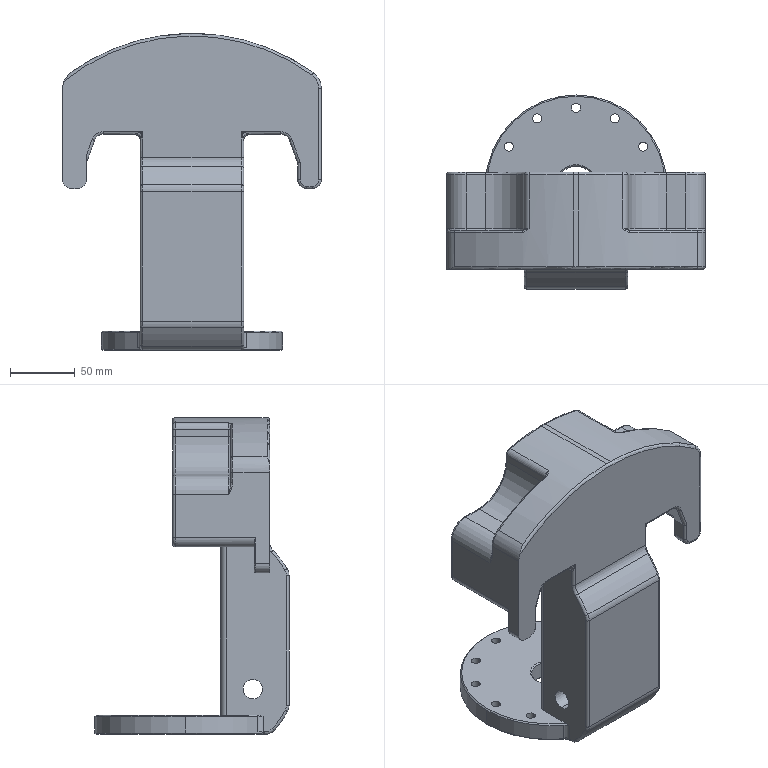Part | SolidWorks | features Fillet 19, ICE 12, MirrorPattern 4, MoveFace 4, Chamfer 3, CirPattern 1, Extrusion 1 | 1 solid | 205 faces | box 200 x 150 x 245 mm | volume 1760406 mm3 | cylinder 101 | torus 48 | plane 30 | spline 14 | cone 12 | commonest cylinder face diameters 4 x25 7 x20 14 x10 10 x9 2 x8 3 x6